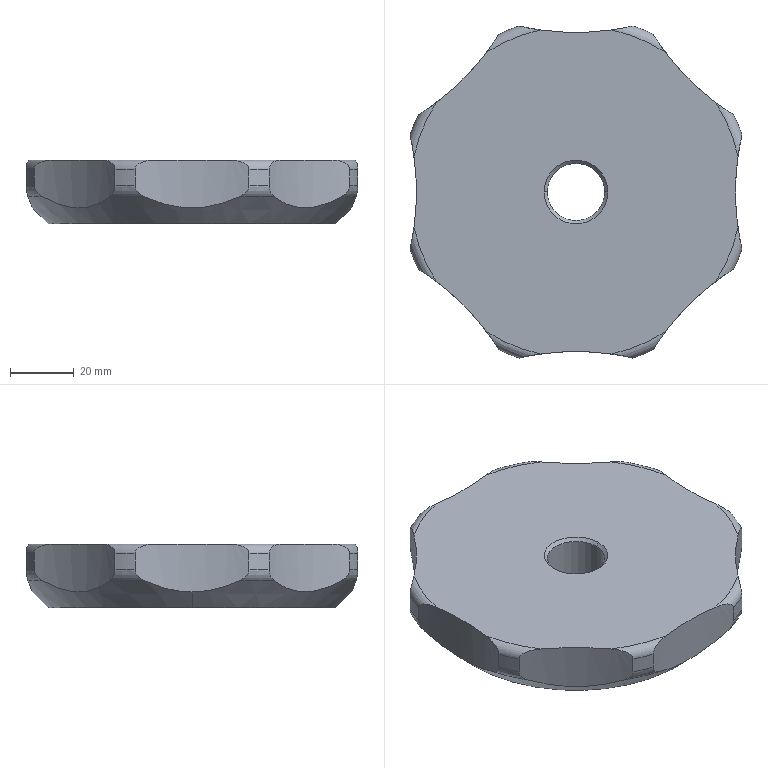Part | STEP file | QA-FC13 | 1 solid | 43 faces | box 104.038 x 104.038 x 20 mm | volume 157045 mm3 | cylinder 19 | torus 16 | cone 6 | plane 2 | commonest cylinder face diameters 160 x9 110 x8 18 x2